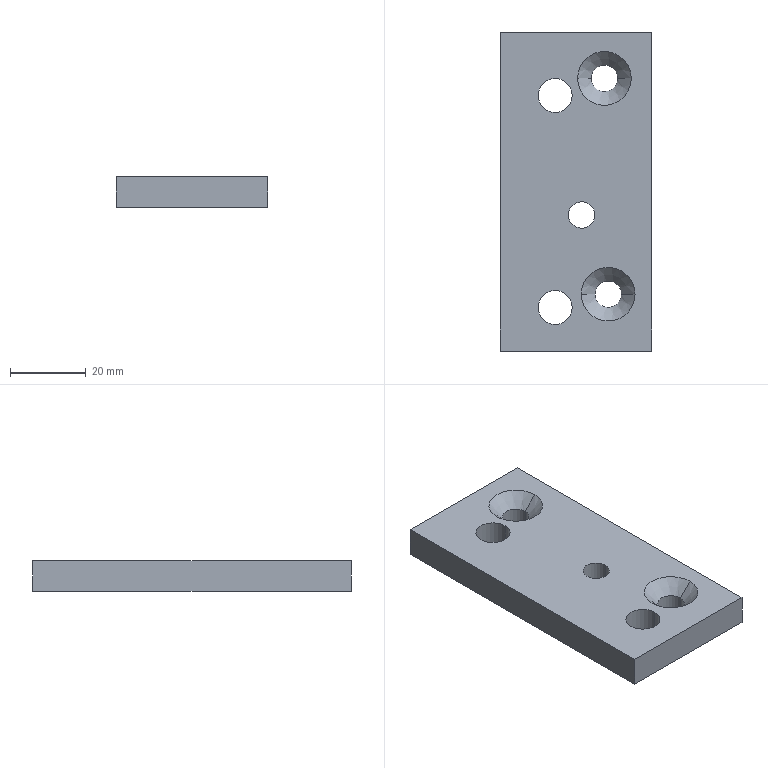Part | 1 solid | 20 faces | box 40 x 84 x 8 mm | volume 24556 mm3 | cylinder 10 | plane 6 | cone 4 | commonest cylinder face diameters 7 x6 9 x4
STEP:
#1=CARTESIAN_POINT('',(0.,0.,0.));
#2=DIRECTION('',(0.,0.,1.));
#3=DIRECTION('',(1.,0.,0.));
#4=AXIS2_PLACEMENT_3D('',#1,#2,#3);
#5=CARTESIAN_POINT('',(-251.148,521.,-248.55));
#6=VERTEX_POINT('',#5);
#7=CARTESIAN_POINT('',(-291.148,521.,-248.55));
#8=VERTEX_POINT('',#7);
#9=CARTESIAN_POINT('',(-251.148,521.,-248.55));
#10=DIRECTION('',(-1.,0.,0.));
#11=VECTOR('',#10,1.);
#12=LINE('',#9,#11);
#13=CARTESIAN_POINT('',(-251.148,521.,-256.55));
#14=DIRECTION('',(0.,1.,0.));
#15=DIRECTION('',(0.,0.,-1.));
#16=AXIS2_PLACEMENT_3D('',#13,#14,#15);
#17=PLANE('',#16);
#18=CARTESIAN_POINT('',(-8.,0.));
#19=DIRECTION('',(0.,1.));
#20=VECTOR('',#19,1.);
#21=LINE('',#18,#20);
#22=(GEOMETRIC_REPRESENTATION_CONTEXT(2)PARAMETRIC_REPRESENTATION_CONTEXT()REPRESENTATION_CONTEXT('',''));
#23=DEFINITIONAL_REPRESENTATION('',(#21),#22);
#24=PCURVE('',#17,#23);
#25=CARTESIAN_POINT('',(-276.648,504.5,-248.55));
#26=DIRECTION('',(0.,0.,1.));
#27=DIRECTION('',(-1.,0.,0.));
#28=AXIS2_PLACEMENT_3D('',#25,#26,#27);
#29=PLANE('',#28);
#30=CARTESIAN_POINT('',(-25.5,-16.5));
#31=DIRECTION('',(1.,0.));
#32=VECTOR('',#31,1.);
#33=LINE('',#30,#32);
#34=(GEOMETRIC_REPRESENTATION_CONTEXT(2)PARAMETRIC_REPRESENTATION_CONTEXT()REPRESENTATION_CONTEXT('',''));
#35=DEFINITIONAL_REPRESENTATION('',(#33),#34);
#36=PCURVE('',#29,#35);
#37=SURFACE_CURVE('',#12,(#24,#36),.PCURVE_S1.);
#38=EDGE_CURVE('',#6,#8,#37,.T.);
#39=ORIENTED_EDGE('',*,*,#38,.F.);
#40=CARTESIAN_POINT('',(-251.148,521.,-256.55));
#41=VERTEX_POINT('',#40);
#42=CARTESIAN_POINT('',(-251.148,521.,-256.55));
#43=DIRECTION('',(0.,0.,1.));
#44=VECTOR('',#43,1.);
#45=LINE('',#42,#44);
#46=CARTESIAN_POINT('',(0.,0.));
#47=DIRECTION('',(-1.,0.));
#48=VECTOR('',#47,1.);
#49=LINE('',#46,#48);
#50=(GEOMETRIC_REPRESENTATION_CONTEXT(2)PARAMETRIC_REPRESENTATION_CONTEXT()REPRESENTATION_CONTEXT('',''));
#51=DEFINITIONAL_REPRESENTATION('',(#49),#50);
#52=PCURVE('',#17,#51);
#53=CARTESIAN_POINT('',(-251.148,437.,-256.55));
#54=DIRECTION('',(1.,0.,0.));
#55=DIRECTION('',(0.,0.,1.));
#56=AXIS2_PLACEMENT_3D('',#53,#54,#55);
#57=PLANE('',#56);
#58=CARTESIAN_POINT('',(0.,-84.));
#59=DIRECTION('',(1.,0.));
#60=VECTOR('',#59,1.);
#61=LINE('',#58,#60);
#62=(GEOMETRIC_REPRESENTATION_CONTEXT(2)PARAMETRIC_REPRESENTATION_CONTEXT()REPRESENTATION_CONTEXT('',''));
#63=DEFINITIONAL_REPRESENTATION('',(#61),#62);
#64=PCURVE('',#57,#63);
#65=SURFACE_CURVE('',#45,(#52,#64),.PCURVE_S1.);
#66=EDGE_CURVE('',#41,#6,#65,.T.);
#67=ORIENTED_EDGE('',*,*,#66,.F.);
#68=CARTESIAN_POINT('',(-291.148,521.,-256.55));
#69=VERTEX_POINT('',#68);
#70=CARTESIAN_POINT('',(-251.148,521.,-256.55));
#71=DIRECTION('',(-1.,0.,0.));
#72=VECTOR('',#71,1.);
#73=LINE('',#70,#72);
#74=CARTESIAN_POINT('',(0.,0.));
#75=DIRECTION('',(0.,1.));
#76=VECTOR('',#75,1.);
#77=LINE('',#74,#76);
#78=(GEOMETRIC_REPRESENTATION_CONTEXT(2)PARAMETRIC_REPRESENTATION_CONTEXT()REPRESENTATION_CONTEXT('',''));
#79=DEFINITIONAL_REPRESENTATION('',(#77),#78);
#80=PCURVE('',#17,#79);
#81=CARTESIAN_POINT('',(-276.648,504.5,-256.55));
#82=DIRECTION('',(0.,0.,1.));
#83=DIRECTION('',(-1.,0.,0.));
#84=AXIS2_PLACEMENT_3D('',#81,#82,#83);
#85=PLANE('',#84);
#86=CARTESIAN_POINT('',(-25.5,-16.5));
#87=DIRECTION('',(1.,0.));
#88=VECTOR('',#87,1.);
#89=LINE('',#86,#88);
#90=(GEOMETRIC_REPRESENTATION_CONTEXT(2)PARAMETRIC_REPRESENTATION_CONTEXT()REPRESENTATION_CONTEXT('',''));
#91=DEFINITIONAL_REPRESENTATION('',(#89),#90);
#92=PCURVE('',#85,#91);
#93=SURFACE_CURVE('',#73,(#80,#92),.PCURVE_S1.);
#94=EDGE_CURVE('',#41,#69,#93,.T.);
#95=ORIENTED_EDGE('',*,*,#94,.T.);
#96=CARTESIAN_POINT('',(-291.148,521.,-256.55));
#97=DIRECTION('',(0.,0.,1.));
#98=VECTOR('',#97,1.);
#99=LINE('',#96,#98);
#100=CARTESIAN_POINT('',(0.,40.));
#101=DIRECTION('',(-1.,0.));
#102=VECTOR('',#101,1.);
#103=LINE('',#100,#102);
#104=(GEOMETRIC_REPRESENTATION_CONTEXT(2)PARAMETRIC_REPRESENTATION_CONTEXT()REPRESENTATION_CONTEXT('',''));
#105=DEFINITIONAL_REPRESENTATION('',(#103),#104);
#106=PCURVE('',#17,#105);
#107=CARTESIAN_POINT('',(-291.148,521.,-256.55));
#108=DIRECTION('',(-1.,0.,0.));
#109=DIRECTION('',(0.,0.,-1.));
#110=AXIS2_PLACEMENT_3D('',#107,#108,#109);
#111=PLANE('',#110);
#112=CARTESIAN_POINT('',(0.,0.));
#113=DIRECTION('',(-1.,0.));
#114=VECTOR('',#113,1.);
#115=LINE('',#112,#114);
#116=(GEOMETRIC_REPRESENTATION_CONTEXT(2)PARAMETRIC_REPRESENTATION_CONTEXT()REPRESENTATION_CONTEXT('',''));
#117=DEFINITIONAL_REPRESENTATION('',(#115),#116);
#118=PCURVE('',#111,#117);
#119=SURFACE_CURVE('',#99,(#106,#118),.PCURVE_S1.);
#120=EDGE_CURVE('',#69,#8,#119,.T.);
#121=ORIENTED_EDGE('',*,*,#120,.T.);
#122=EDGE_LOOP('',(#39,#67,#95,#121));
#123=FACE_BOUND('',#122,.T.);
#124=ADVANCED_FACE('',(#123),#17,.T.);
#125=CARTESIAN_POINT('',(-291.148,437.,-248.55));
#126=VERTEX_POINT('',#125);
#127=CARTESIAN_POINT('',(-291.148,521.,-248.55));
#128=DIRECTION('',(0.,-1.,0.));
#129=VECTOR('',#128,1.);
#130=LINE('',#127,#129);
#131=CARTESIAN_POINT('',(-8.,0.));
#132=DIRECTION('',(0.,1.));
#133=VECTOR('',#132,1.);
#134=LINE('',#131,#133);
#135=(GEOMETRIC_REPRESENTATION_CONTEXT(2)PARAMETRIC_REPRESENTATION_CONTEXT()REPRESENTATION_CONTEXT('',''));
#136=DEFINITIONAL_REPRESENTATION('',(#134),#135);
#137=PCURVE('',#111,#136);
#138=CARTESIAN_POINT('',(14.5,-16.5));
#139=DIRECTION('',(0.,1.));
#140=VECTOR('',#139,1.);
#141=LINE('',#138,#140);
#142=(GEOMETRIC_REPRESENTATION_CONTEXT(2)PARAMETRIC_REPRESENTATION_CONTEXT()REPRESENTATION_CONTEXT('',''));
#143=DEFINITIONAL_REPRESENTATION('',(#141),#142);
#144=PCURVE('',#29,#143);
#145=SURFACE_CURVE('',#130,(#137,#144),.PCURVE_S1.);
#146=EDGE_CURVE('',#8,#126,#145,.T.);
#147=ORIENTED_EDGE('',*,*,#146,.F.);
#148=ORIENTED_EDGE('',*,*,#120,.F.);
#149=CARTESIAN_POINT('',(-291.148,437.,-256.55));
#150=VERTEX_POINT('',#149);
#151=CARTESIAN_POINT('',(-291.148,521.,-256.55));
#152=DIRECTION('',(0.,-1.,0.));
#153=VECTOR('',#152,1.);
#154=LINE('',#151,#153);
#155=CARTESIAN_POINT('',(0.,0.));
#156=DIRECTION('',(0.,1.));
#157=VECTOR('',#156,1.);
#158=LINE('',#155,#157);
#159=(GEOMETRIC_REPRESENTATION_CONTEXT(2)PARAMETRIC_REPRESENTATION_CONTEXT()REPRESENTATION_CONTEXT('',''));
#160=DEFINITIONAL_REPRESENTATION('',(#158),#159);
#161=PCURVE('',#111,#160);
#162=CARTESIAN_POINT('',(14.5,-16.5));
#163=DIRECTION('',(0.,1.));
#164=VECTOR('',#163,1.);
#165=LINE('',#162,#164);
#166=(GEOMETRIC_REPRESENTATION_CONTEXT(2)PARAMETRIC_REPRESENTATION_CONTEXT()REPRESENTATION_CONTEXT('',''));
#167=DEFINITIONAL_REPRESENTATION('',(#165),#166);
#168=PCURVE('',#85,#167);
#169=SURFACE_CURVE('',#154,(#161,#168),.PCURVE_S1.);
#170=EDGE_CURVE('',#69,#150,#169,.T.);
#171=ORIENTED_EDGE('',*,*,#170,.T.);
#172=CARTESIAN_POINT('',(-291.148,437.,-256.55));
#173=DIRECTION('',(0.,0.,1.));
#174=VECTOR('',#173,1.);
#175=LINE('',#172,#174);
#176=CARTESIAN_POINT('',(0.,84.));
#177=DIRECTION('',(-1.,0.));
#178=VECTOR('',#177,1.);
#179=LINE('',#176,#178);
#180=(GEOMETRIC_REPRESENTATION_CONTEXT(2)PARAMETRIC_REPRESENTATION_CONTEXT()REPRESENTATION_CONTEXT('',''));
#181=DEFINITIONAL_REPRESENTATION('',(#179),#180);
#182=PCURVE('',#111,#181);
#183=CARTESIAN_POINT('',(-291.148,437.,-256.55));
#184=DIRECTION('',(0.,-1.,0.));
#185=DIRECTION('',(0.,0.,1.));
#186=AXIS2_PLACEMENT_3D('',#183,#184,#185);
#187=PLANE('',#186);
#188=CARTESIAN_POINT('',(0.,0.));
#189=DIRECTION('',(1.,0.));
#190=VECTOR('',#189,1.);
#191=LINE('',#188,#190);
#192=(GEOMETRIC_REPRESENTATION_CONTEXT(2)PARAMETRIC_REPRESENTATION_CONTEXT()REPRESENTATION_CONTEXT('',''));
#193=DEFINITIONAL_REPRESENTATION('',(#191),#192);
#194=PCURVE('',#187,#193);
#195=SURFACE_CURVE('',#175,(#182,#194),.PCURVE_S1.);
#196=EDGE_CURVE('',#150,#126,#195,.T.);
#197=ORIENTED_EDGE('',*,*,#196,.T.);
#198=EDGE_LOOP('',(#147,#148,#171,#197));
#199=FACE_BOUND('',#198,.T.);
#200=ADVANCED_FACE('',(#199),#111,.T.);
#201=CARTESIAN_POINT('',(-251.148,437.,-248.55));
#202=VERTEX_POINT('',#201);
#203=CARTESIAN_POINT('',(-291.148,437.,-248.55));
#204=DIRECTION('',(1.,0.,0.));
#205=VECTOR('',#204,1.);
#206=LINE('',#203,#205);
#207=CARTESIAN_POINT('',(8.,0.));
#208=DIRECTION('',(0.,-1.));
#209=VECTOR('',#208,1.);
#210=LINE('',#207,#209);
#211=(GEOMETRIC_REPRESENTATION_CONTEXT(2)PARAMETRIC_REPRESENTATION_CONTEXT()REPRESENTATION_CONTEXT('',''));
#212=DEFINITIONAL_REPRESENTATION('',(#210),#211);
#213=PCURVE('',#187,#212);
#214=CARTESIAN_POINT('',(14.5,67.5));
#215=DIRECTION('',(-1.,0.));
#216=VECTOR('',#215,1.);
#217=LINE('',#214,#216);
#218=(GEOMETRIC_REPRESENTATION_CONTEXT(2)PARAMETRIC_REPRESENTATION_CONTEXT()REPRESENTATION_CONTEXT('',''));
#219=DEFINITIONAL_REPRESENTATION('',(#217),#218);
#220=PCURVE('',#29,#219);
#221=SURFACE_CURVE('',#206,(#213,#220),.PCURVE_S1.);
#222=EDGE_CURVE('',#126,#202,#221,.T.);
#223=ORIENTED_EDGE('',*,*,#222,.F.);
#224=ORIENTED_EDGE('',*,*,#196,.F.);
#225=CARTESIAN_POINT('',(-251.148,437.,-256.55));
#226=VERTEX_POINT('',#225);
#227=CARTESIAN_POINT('',(-291.148,437.,-256.55));
#228=DIRECTION('',(1.,0.,0.));
#229=VECTOR('',#228,1.);
#230=LINE('',#227,#229);
#231=CARTESIAN_POINT('',(0.,0.));
#232=DIRECTION('',(0.,-1.));
#233=VECTOR('',#232,1.);
#234=LINE('',#231,#233);
#235=(GEOMETRIC_REPRESENTATION_CONTEXT(2)PARAMETRIC_REPRESENTATION_CONTEXT()REPRESENTATION_CONTEXT('',''));
#236=DEFINITIONAL_REPRESENTATION('',(#234),#235);
#237=PCURVE('',#187,#236);
#238=CARTESIAN_POINT('',(14.5,67.5));
#239=DIRECTION('',(-1.,0.));
#240=VECTOR('',#239,1.);
#241=LINE('',#238,#240);
#242=(GEOMETRIC_REPRESENTATION_CONTEXT(2)PARAMETRIC_REPRESENTATION_CONTEXT()REPRESENTATION_CONTEXT('',''));
#243=DEFINITIONAL_REPRESENTATION('',(#241),#242);
#244=PCURVE('',#85,#243);
#245=SURFACE_CURVE('',#230,(#237,#244),.PCURVE_S1.);
#246=EDGE_CURVE('',#150,#226,#245,.T.);
#247=ORIENTED_EDGE('',*,*,#246,.T.);
#248=CARTESIAN_POINT('',(-251.148,437.,-256.55));
#249=DIRECTION('',(0.,0.,1.));
#250=VECTOR('',#249,1.);
#251=LINE('',#248,#250);
#252=CARTESIAN_POINT('',(0.,-40.));
#253=DIRECTION('',(1.,0.));
#254=VECTOR('',#253,1.);
#255=LINE('',#252,#254);
#256=(GEOMETRIC_REPRESENTATION_CONTEXT(2)PARAMETRIC_REPRESENTATION_CONTEXT()REPRESENTATION_CONTEXT('',''));
#257=DEFINITIONAL_REPRESENTATION('',(#255),#256);
#258=PCURVE('',#187,#257);
#259=CARTESIAN_POINT('',(0.,0.));
#260=DIRECTION('',(1.,0.));
#261=VECTOR('',#260,1.);
#262=LINE('',#259,#261);
#263=(GEOMETRIC_REPRESENTATION_CONTEXT(2)PARAMETRIC_REPRESENTATION_CONTEXT()REPRESENTATION_CONTEXT('',''));
#264=DEFINITIONAL_REPRESENTATION('',(#262),#263);
#265=PCURVE('',#57,#264);
#266=SURFACE_CURVE('',#251,(#258,#265),.PCURVE_S1.);
#267=EDGE_CURVE('',#226,#202,#266,.T.);
#268=ORIENTED_EDGE('',*,*,#267,.T.);
#269=EDGE_LOOP('',(#223,#224,#247,#268));
#270=FACE_BOUND('',#269,.T.);
#271=ADVANCED_FACE('',(#270),#187,.T.);
#272=CARTESIAN_POINT('',(-251.148,437.,-248.55));
#273=DIRECTION('',(0.,1.,0.));
#274=VECTOR('',#273,1.);
#275=LINE('',#272,#274);
#276=CARTESIAN_POINT('',(8.,0.));
#277=DIRECTION('',(0.,-1.));
#278=VECTOR('',#277,1.);
#279=LINE('',#276,#278);
#280=(GEOMETRIC_REPRESENTATION_CONTEXT(2)PARAMETRIC_REPRESENTATION_CONTEXT()REPRESENTATION_CONTEXT('',''));
#281=DEFINITIONAL_REPRESENTATION('',(#279),#280);
#282=PCURVE('',#57,#281);
#283=CARTESIAN_POINT('',(-25.5,67.5));
#284=DIRECTION('',(0.,-1.));
#285=VECTOR('',#284,1.);
#286=LINE('',#283,#285);
#287=(GEOMETRIC_REPRESENTATION_CONTEXT(2)PARAMETRIC_REPRESENTATION_CONTEXT()REPRESENTATION_CONTEXT('',''));
#288=DEFINITIONAL_REPRESENTATION('',(#286),#287);
#289=PCURVE('',#29,#288);
#290=SURFACE_CURVE('',#275,(#282,#289),.PCURVE_S1.);
#291=EDGE_CURVE('',#202,#6,#290,.T.);
#292=ORIENTED_EDGE('',*,*,#291,.F.);
#293=ORIENTED_EDGE('',*,*,#267,.F.);
#294=CARTESIAN_POINT('',(-251.148,437.,-256.55));
#295=DIRECTION('',(0.,1.,0.));
#296=VECTOR('',#295,1.);
#297=LINE('',#294,#296);
#298=CARTESIAN_POINT('',(0.,0.));
#299=DIRECTION('',(0.,-1.));
#300=VECTOR('',#299,1.);
#301=LINE('',#298,#300);
#302=(GEOMETRIC_REPRESENTATION_CONTEXT(2)PARAMETRIC_REPRESENTATION_CONTEXT()REPRESENTATION_CONTEXT('',''));
#303=DEFINITIONAL_REPRESENTATION('',(#301),#302);
#304=PCURVE('',#57,#303);
#305=CARTESIAN_POINT('',(-25.5,67.5));
#306=DIRECTION('',(0.,-1.));
#307=VECTOR('',#306,1.);
#308=LINE('',#305,#307);
#309=(GEOMETRIC_REPRESENTATION_CONTEXT(2)PARAMETRIC_REPRESENTATION_CONTEXT()REPRESENTATION_CONTEXT('',''));
#310=DEFINITIONAL_REPRESENTATION('',(#308),#309);
#311=PCURVE('',#85,#310);
#312=SURFACE_CURVE('',#297,(#304,#311),.PCURVE_S1.);
#313=EDGE_CURVE('',#226,#41,#312,.T.);
#314=ORIENTED_EDGE('',*,*,#313,.T.);
#315=ORIENTED_EDGE('',*,*,#66,.T.);
#316=EDGE_LOOP('',(#292,#293,#314,#315));
#317=FACE_BOUND('',#316,.T.);
#318=ADVANCED_FACE('',(#317),#57,.T.);
#319=CARTESIAN_POINT('',(-259.148,452.,-256.55));
#320=VERTEX_POINT('',#319);
#321=CARTESIAN_POINT('',(-266.148,452.,-256.55));
#322=VERTEX_POINT('',#321);
#323=CARTESIAN_POINT('',(-262.648,452.,-256.55));
#324=DIRECTION('',(0.,0.,1.));
#325=DIRECTION('',(1.,0.,0.));
#326=AXIS2_PLACEMENT_3D('',#323,#324,#325);
#327=CIRCLE('',#326,3.5);
#328=CARTESIAN_POINT('',(-14.,52.5));
#329=DIRECTION('',(-1.,0.));
#330=AXIS2_PLACEMENT_2D('',#328,#329);
#331=CIRCLE('',#330,3.5);
#332=(GEOMETRIC_REPRESENTATION_CONTEXT(2)PARAMETRIC_REPRESENTATION_CONTEXT()REPRESENTATION_CONTEXT('',''));
#333=DEFINITIONAL_REPRESENTATION('',(#331),#332);
#334=PCURVE('',#85,#333);
#335=CARTESIAN_POINT('',(-262.648,452.,-298.55));
#336=DIRECTION('',(0.,0.,-1.));
#337=DIRECTION('',(0.,-1.,0.));
#338=AXIS2_PLACEMENT_3D('',#335,#336,#337);
#339=CYLINDRICAL_SURFACE('',#338,3.5);
#340=CARTESIAN_POINT('',(4.712,-42.));
#341=DIRECTION('',(-1.,0.));
#342=VECTOR('',#341,1.);
#343=LINE('',#340,#342);
#344=(GEOMETRIC_REPRESENTATION_CONTEXT(2)PARAMETRIC_REPRESENTATION_CONTEXT()REPRESENTATION_CONTEXT('',''));
#345=DEFINITIONAL_REPRESENTATION('',(#343),#344);
#346=PCURVE('',#339,#345);
#347=SURFACE_CURVE('',#327,(#334,#346),.PCURVE_S1.);
#348=EDGE_CURVE('',#320,#322,#347,.T.);
#349=ORIENTED_EDGE('',*,*,#348,.T.);
#350=CARTESIAN_POINT('',(-262.648,452.,-256.55));
#351=DIRECTION('',(0.,0.,1.));
#352=DIRECTION('',(1.,0.,0.));
#353=AXIS2_PLACEMENT_3D('',#350,#351,#352);
#354=CIRCLE('',#353,3.5);
#355=CARTESIAN_POINT('',(-14.,52.5));
#356=DIRECTION('',(-1.,0.));
#357=AXIS2_PLACEMENT_2D('',#355,#356);
#358=CIRCLE('',#357,3.5);
#359=(GEOMETRIC_REPRESENTATION_CONTEXT(2)PARAMETRIC_REPRESENTATION_CONTEXT()REPRESENTATION_CONTEXT('',''));
#360=DEFINITIONAL_REPRESENTATION('',(#358),#359);
#361=PCURVE('',#85,#360);
#362=CARTESIAN_POINT('',(-262.648,452.,-298.55));
#363=DIRECTION('',(0.,0.,-1.));
#364=DIRECTION('',(0.,1.,0.));
#365=AXIS2_PLACEMENT_3D('',#362,#363,#364);
#366=CYLINDRICAL_SURFACE('',#365,3.5);
#367=CARTESIAN_POINT('',(7.854,-42.));
#368=DIRECTION('',(-1.,0.));
#369=VECTOR('',#368,1.);
#370=LINE('',#367,#369);
#371=(GEOMETRIC_REPRESENTATION_CONTEXT(2)PARAMETRIC_REPRESENTATION_CONTEXT()REPRESENTATION_CONTEXT('',''));
#372=DEFINITIONAL_REPRESENTATION('',(#370),#371);
#373=PCURVE('',#366,#372);
#374=SURFACE_CURVE('',#354,(#361,#373),.PCURVE_S1.);
#375=EDGE_CURVE('',#322,#320,#374,.T.);
#376=ORIENTED_EDGE('',*,*,#375,.T.);
#377=EDGE_LOOP('',(#349,#376));
#378=FACE_BOUND('',#377,.T.);
#379=CARTESIAN_POINT('',(-260.148,509.,-256.55));
#380=VERTEX_POINT('',#379);
#381=CARTESIAN_POINT('',(-267.148,509.,-256.55));
#382=VERTEX_POINT('',#381);
#383=CARTESIAN_POINT('',(-263.648,509.,-256.55));
#384=DIRECTION('',(0.,0.,1.));
#385=DIRECTION('',(1.,0.,0.));
#386=AXIS2_PLACEMENT_3D('',#383,#384,#385);
#387=CIRCLE('',#386,3.5);
#388=CARTESIAN_POINT('',(-13.,-4.5));
#389=DIRECTION('',(-1.,0.));
#390=AXIS2_PLACEMENT_2D('',#388,#389);
#391=CIRCLE('',#390,3.5);
#392=(GEOMETRIC_REPRESENTATION_CONTEXT(2)PARAMETRIC_REPRESENTATION_CONTEXT()REPRESENTATION_CONTEXT('',''));
#393=DEFINITIONAL_REPRESENTATION('',(#391),#392);
#394=PCURVE('',#85,#393);
#395=CARTESIAN_POINT('',(-263.648,509.,-298.55));
#396=DIRECTION('',(0.,0.,-1.));
#397=DIRECTION('',(0.,-1.,0.));
#398=AXIS2_PLACEMENT_3D('',#395,#396,#397);
#399=CYLINDRICAL_SURFACE('',#398,3.5);
#400=CARTESIAN_POINT('',(4.712,-42.));
#401=DIRECTION('',(-1.,0.));
#402=VECTOR('',#401,1.);
#403=LINE('',#400,#402);
#404=(GEOMETRIC_REPRESENTATION_CONTEXT(2)PARAMETRIC_REPRESENTATION_CONTEXT()REPRESENTATION_CONTEXT('',''));
#405=DEFINITIONAL_REPRESENTATION('',(#403),#404);
#406=PCURVE('',#399,#405);
#407=SURFACE_CURVE('',#387,(#394,#406),.PCURVE_S1.);
#408=EDGE_CURVE('',#380,#382,#407,.T.);
#409=ORIENTED_EDGE('',*,*,#408,.T.);
#410=CARTESIAN_POINT('',(-263.648,509.,-256.55));
#411=DIRECTION('',(0.,0.,1.));
#412=DIRECTION('',(1.,0.,0.));
#413=AXIS2_PLACEMENT_3D('',#410,#411,#412);
#414=CIRCLE('',#413,3.5);
#415=CARTESIAN_POINT('',(-13.,-4.5));
#416=DIRECTION('',(-1.,0.));
#417=AXIS2_PLACEMENT_2D('',#415,#416);
#418=CIRCLE('',#417,3.5);
#419=(GEOMETRIC_REPRESENTATION_CONTEXT(2)PARAMETRIC_REPRESENTATION_CONTEXT()REPRESENTATION_CONTEXT('',''));
#420=DEFINITIONAL_REPRESENTATION('',(#418),#419);
#421=PCURVE('',#85,#420);
#422=CARTESIAN_POINT('',(-263.648,509.,-298.55));
#423=DIRECTION('',(0.,0.,-1.));
#424=DIRECTION('',(0.,1.,0.));
#425=AXIS2_PLACEMENT_3D('',#422,#423,#424);
#426=CYLINDRICAL_SURFACE('',#425,3.5);
#427=CARTESIAN_POINT('',(7.854,-42.));
#428=DIRECTION('',(-1.,0.));
#429=VECTOR('',#428,1.);
#430=LINE('',#427,#429);
#431=(GEOMETRIC_REPRESENTATION_CONTEXT(2)PARAMETRIC_REPRESENTATION_CONTEXT()REPRESENTATION_CONTEXT('',''));
#432=DEFINITIONAL_REPRESENTATION('',(#430),#431);
#433=PCURVE('',#426,#432);
#434=SURFACE_CURVE('',#414,(#421,#433),.PCURVE_S1.);
#435=EDGE_CURVE('',#382,#380,#434,.T.);
#436=ORIENTED_EDGE('',*,*,#435,.T.);
#437=EDGE_LOOP('',(#409,#436));
#438=FACE_BOUND('',#437,.T.);
#439=ORIENTED_EDGE('',*,*,#94,.F.);
#440=ORIENTED_EDGE('',*,*,#313,.F.);
#441=ORIENTED_EDGE('',*,*,#246,.F.);
#442=ORIENTED_EDGE('',*,*,#170,.F.);
#443=EDGE_LOOP('',(#439,#440,#441,#442));
#444=FACE_BOUND('',#443,.T.);
#445=CARTESIAN_POINT('',(-281.148,504.5,-256.55));
#446=VERTEX_POINT('',#445);
#447=CARTESIAN_POINT('',(-272.148,504.5,-256.55));
#448=VERTEX_POINT('',#447);
#449=CARTESIAN_POINT('',(-276.648,504.5,-256.55));
#450=DIRECTION('',(0.,0.,1.));
#451=DIRECTION('',(-1.,0.,0.));
#452=AXIS2_PLACEMENT_3D('',#449,#450,#451);
#453=CIRCLE('',#452,4.5);
#454=CARTESIAN_POINT('',(0.,0.));
#455=DIRECTION('',(1.,0.));
#456=AXIS2_PLACEMENT_2D('',#454,#455);
#457=CIRCLE('',#456,4.5);
#458=(GEOMETRIC_REPRESENTATION_CONTEXT(2)PARAMETRIC_REPRESENTATION_CONTEXT()REPRESENTATION_CONTEXT('',''));
#459=DEFINITIONAL_REPRESENTATION('',(#457),#458);
#460=PCURVE('',#85,#459);
#461=CARTESIAN_POINT('',(-276.648,504.5,-256.55));
#462=DIRECTION('',(0.,0.,1.));
#463=DIRECTION('',(0.,1.,0.));
#464=AXIS2_PLACEMENT_3D('',#461,#462,#463);
#465=CYLINDRICAL_SURFACE('',#464,4.5);
#466=CARTESIAN_POINT('',(1.571,0.));
#467=DIRECTION('',(1.,0.));
#468=VECTOR('',#467,1.);
#469=LINE('',#466,#468);
#470=(GEOMETRIC_REPRESENTATION_CONTEXT(2)PARAMETRIC_REPRESENTATION_CONTEXT()REPRESENTATION_CONTEXT('',''));
#471=DEFINITIONAL_REPRESENTATION('',(#469),#470);
#472=PCURVE('',#465,#471);
#473=SURFACE_CURVE('',#453,(#460,#472),.PCURVE_S1.);
#474=EDGE_CURVE('',#446,#448,#473,.T.);
#475=ORIENTED_EDGE('',*,*,#474,.T.);
#476=CARTESIAN_POINT('',(-276.648,504.5,-256.55));
#477=DIRECTION('',(0.,0.,1.));
#478=DIRECTION('',(-1.,0.,0.));
#479=AXIS2_PLACEMENT_3D('',#476,#477,#478);
#480=CIRCLE('',#479,4.5);
#481=CARTESIAN_POINT('',(0.,0.));
#482=DIRECTION('',(1.,0.));
#483=AXIS2_PLACEMENT_2D('',#481,#482);
#484=CIRCLE('',#483,4.5);
#485=(GEOMETRIC_REPRESENTATION_CONTEXT(2)PARAMETRIC_REPRESENTATION_CONTEXT()REPRESENTATION_CONTEXT('',''));
#486=DEFINITIONAL_REPRESENTATION('',(#484),#485);
#487=PCURVE('',#85,#486);
#488=CARTESIAN_POINT('',(-276.648,504.5,-256.55));
#489=DIRECTION('',(0.,0.,1.));
#490=DIRECTION('',(0.,-1.,0.));
#491=AXIS2_PLACEMENT_3D('',#488,#489,#490);
#492=CYLINDRICAL_SURFACE('',#491,4.5);
#493=CARTESIAN_POINT('',(-1.571,0.));
#494=DIRECTION('',(1.,0.));
#495=VECTOR('',#494,1.);
#496=LINE('',#493,#495);
#497=(GEOMETRIC_REPRESENTATION_CONTEXT(2)PARAMETRIC_REPRESENTATION_CONTEXT()REPRESENTATION_CONTEXT('',''));
#498=DEFINITIONAL_REPRESENTATION('',(#496),#497);
#499=PCURVE('',#492,#498);
#500=SURFACE_CURVE('',#480,(#487,#499),.PCURVE_S1.);
#501=EDGE_CURVE('',#448,#446,#500,.T.);
#502=ORIENTED_EDGE('',*,*,#501,.T.);
#503=EDGE_LOOP('',(#475,#502));
#504=FACE_BOUND('',#503,.T.);
#505=CARTESIAN_POINT('',(-273.148,472.924,-256.55));
#506=VERTEX_POINT('',#505);
#507=CARTESIAN_POINT('',(-266.148,472.924,-256.55));
#508=VERTEX_POINT('',#507);
#509=CARTESIAN_POINT('',(-269.648,472.924,-256.55));
#510=DIRECTION('',(0.,0.,1.));
#511=DIRECTION('',(-1.,0.,0.));
#512=AXIS2_PLACEMENT_3D('',#509,#510,#511);
#513=CIRCLE('',#512,3.5);
#514=CARTESIAN_POINT('',(-7.,31.576));
#515=DIRECTION('',(1.,0.));
#516=AXIS2_PLACEMENT_2D('',#514,#515);
#517=CIRCLE('',#516,3.5);
#518=(GEOMETRIC_REPRESENTATION_CONTEXT(2)PARAMETRIC_REPRESENTATION_CONTEXT()REPRESENTATION_CONTEXT('',''));
#519=DEFINITIONAL_REPRESENTATION('',(#517),#518);
#520=PCURVE('',#85,#519);
#521=CARTESIAN_POINT('',(-269.648,472.924,-256.55));
#522=DIRECTION('',(0.,0.,1.));
#523=DIRECTION('',(0.,1.,0.));
#524=AXIS2_PLACEMENT_3D('',#521,#522,#523);
#525=CYLINDRICAL_SURFACE('',#524,3.5);
#526=CARTESIAN_POINT('',(1.571,0.));
#527=DIRECTION('',(1.,0.));
#528=VECTOR('',#527,1.);
#529=LINE('',#526,#528);
#530=(GEOMETRIC_REPRESENTATION_CONTEXT(2)PARAMETRIC_REPRESENTATION_CONTEXT()REPRESENTATION_CONTEXT('',''));
#531=DEFINITIONAL_REPRESENTATION('',(#529),#530);
#532=PCURVE('',#525,#531);
#533=SURFACE_CURVE('',#513,(#520,#532),.PCURVE_S1.);
#534=EDGE_CURVE('',#506,#508,#533,.T.);
#535=ORIENTED_EDGE('',*,*,#534,.T.);
#536=CARTESIAN_POINT('',(-269.648,472.924,-256.55));
#537=DIRECTION('',(0.,0.,1.));
#538=DIRECTION('',(-1.,0.,0.));
#539=AXIS2_PLACEMENT_3D('',#536,#537,#538);
#540=CIRCLE('',#539,3.5);
#541=CARTESIAN_POINT('',(-7.,31.576));
#542=DIRECTION('',(1.,0.));
#543=AXIS2_PLACEMENT_2D('',#541,#542);
#544=CIRCLE('',#543,3.5);
#545=(GEOMETRIC_REPRESENTATION_CONTEXT(2)PARAMETRIC_REPRESENTATION_CONTEXT()REPRESENTATION_CONTEXT('',''));
#546=DEFINITIONAL_REPRESENTATION('',(#544),#545);
#547=PCURVE('',#85,#546);
#548=CARTESIAN_POINT('',(-269.648,472.924,-256.55));
#549=DIRECTION('',(0.,0.,1.));
#550=DIRECTION('',(0.,-1.,0.));
#551=AXIS2_PLACEMENT_3D('',#548,#549,#550);
#552=CYLINDRICAL_SURFACE('',#551,3.5);
#553=CARTESIAN_POINT('',(-1.571,0.));
#554=DIRECTION('',(1.,0.));
#555=VECTOR('',#554,1.);
#556=LINE('',#553,#555);
#557=(GEOMETRIC_REPRESENTATION_CONTEXT(2)PARAMETRIC_REPRESENTATION_CONTEXT()REPRESENTATION_CONTEXT('',''));
#558=DEFINITIONAL_REPRESENTATION('',(#556),#557);
#559=PCURVE('',#552,#558);
#560=SURFACE_CURVE('',#540,(#547,#559),.PCURVE_S1.);
#561=EDGE_CURVE('',#508,#506,#560,.T.);
#562=ORIENTED_EDGE('',*,*,#561,.T.);
#563=EDGE_LOOP('',(#535,#562));
#564=FACE_BOUND('',#563,.T.);
#565=CARTESIAN_POINT('',(-281.148,448.5,-256.55));
#566=VERTEX_POINT('',#565);
#567=CARTESIAN_POINT('',(-272.148,448.5,-256.55));
#568=VERTEX_POINT('',#567);
#569=CARTESIAN_POINT('',(-276.648,448.5,-256.55));
#570=DIRECTION('',(0.,0.,1.));
#571=DIRECTION('',(-1.,0.,0.));
#572=AXIS2_PLACEMENT_3D('',#569,#570,#571);
#573=CIRCLE('',#572,4.5);
#574=CARTESIAN_POINT('',(0.,56.));
#575=DIRECTION('',(1.,0.));
#576=AXIS2_PLACEMENT_2D('',#574,#575);
#577=CIRCLE('',#576,4.5);
#578=(GEOMETRIC_REPRESENTATION_CONTEXT(2)PARAMETRIC_REPRESENTATION_CONTEXT()REPRESENTATION_CONTEXT('',''));
#579=DEFINITIONAL_REPRESENTATION('',(#577),#578);
#580=PCURVE('',#85,#579);
#581=CARTESIAN_POINT('',(-276.648,448.5,-256.55));
#582=DIRECTION('',(0.,0.,1.));
#583=DIRECTION('',(0.,1.,0.));
#584=AXIS2_PLACEMENT_3D('',#581,#582,#583);
#585=CYLINDRICAL_SURFACE('',#584,4.5);
#586=CARTESIAN_POINT('',(1.571,0.));
#587=DIRECTION('',(1.,0.));
#588=VECTOR('',#587,1.);
#589=LINE('',#586,#588);
#590=(GEOMETRIC_REPRESENTATION_CONTEXT(2)PARAMETRIC_REPRESENTATION_CONTEXT()REPRESENTATION_CONTEXT('',''));
#591=DEFINITIONAL_REPRESENTATION('',(#589),#590);
#592=PCURVE('',#585,#591);
#593=SURFACE_CURVE('',#573,(#580,#592),.PCURVE_S1.);
#594=EDGE_CURVE('',#566,#568,#593,.T.);
#595=ORIENTED_EDGE('',*,*,#594,.T.);
#596=CARTESIAN_POINT('',(-276.648,448.5,-256.55));
#597=DIRECTION('',(0.,0.,1.));
#598=DIRECTION('',(-1.,0.,0.));
#599=AXIS2_PLACEMENT_3D('',#596,#597,#598);
#600=CIRCLE('',#599,4.5);
#601=CARTESIAN_POINT('',(0.,56.));
#602=DIRECTION('',(1.,0.));
#603=AXIS2_PLACEMENT_2D('',#601,#602);
#604=CIRCLE('',#603,4.5);
#605=(GEOMETRIC_REPRESENTATION_CONTEXT(2)PARAMETRIC_REPRESENTATION_CONTEXT()REPRESENTATION_CONTEXT('',''));
#606=DEFINITIONAL_REPRESENTATION('',(#604),#605);
#607=PCURVE('',#85,#606);
#608=CARTESIAN_POINT('',(-276.648,448.5,-256.55));
#609=DIRECTION('',(0.,0.,1.));
#610=DIRECTION('',(0.,-1.,0.));
#611=AXIS2_PLACEMENT_3D('',#608,#609,#610);
#612=CYLINDRICAL_SURFACE('',#611,4.5);
#613=CARTESIAN_POINT('',(-1.571,0.));
#614=DIRECTION('',(1.,0.));
#615=VECTOR('',#614,1.);
#616=LINE('',#613,#615);
#617=(GEOMETRIC_REPRESENTATION_CONTEXT(2)PARAMETRIC_REPRESENTATION_CONTEXT()REPRESENTATION_CONTEXT('',''));
#618=DEFINITIONAL_REPRESENTATION('',(#616),#617);
#619=PCURVE('',#612,#618);
#620=SURFACE_CURVE('',#600,(#607,#619),.PCURVE_S1.);
#621=EDGE_CURVE('',#568,#566,#620,.T.);
#622=ORIENTED_EDGE('',*,*,#621,.T.);
#623=EDGE_LOOP('',(#595,#622));
#624=FACE_BOUND('',#623,.T.);
#625=ADVANCED_FACE('',(#378,#438,#444,#504,#564,#624),#85,.F.);
#626=ORIENTED_EDGE('',*,*,#621,.T.);
#627=CARTESIAN_POINT('',(-281.148,448.5,-248.55));
#628=VERTEX_POINT('',#627);
#629=CARTESIAN_POINT('',(-281.148,448.5,-256.55));
#630=DIRECTION('',(0.,0.,1.));
#631=VECTOR('',#630,1.);
#632=LINE('',#629,#631);
#633=CARTESIAN_POINT('',(4.712,0.));
#634=DIRECTION('',(0.,1.));
#635=VECTOR('',#634,1.);
#636=LINE('',#633,#635);
#637=(GEOMETRIC_REPRESENTATION_CONTEXT(2)PARAMETRIC_REPRESENTATION_CONTEXT()REPRESENTATION_CONTEXT('',''));
#638=DEFINITIONAL_REPRESENTATION('',(#636),#637);
#639=PCURVE('',#612,#638);
#640=CARTESIAN_POINT('',(1.571,0.));
#641=DIRECTION('',(0.,1.));
#642=VECTOR('',#641,1.);
#643=LINE('',#640,#642);
#644=(GEOMETRIC_REPRESENTATION_CONTEXT(2)PARAMETRIC_REPRESENTATION_CONTEXT()REPRESENTATION_CONTEXT('',''));
#645=DEFINITIONAL_REPRESENTATION('',(#643),#644);
#646=PCURVE('',#585,#645);
#647=SURFACE_CURVE('',#632,(#639,#646),.PCURVE_S1.);
#648=EDGE_CURVE('',#566,#628,#647,.T.);
#649=ORIENTED_EDGE('',*,*,#648,.T.);
#650=CARTESIAN_POINT('',(-272.148,448.5,-248.55));
#651=VERTEX_POINT('',#650);
#652=CARTESIAN_POINT('',(-276.648,448.5,-248.55));
#653=DIRECTION('',(0.,0.,1.));
#654=DIRECTION('',(-1.,0.,0.));
#655=AXIS2_PLACEMENT_3D('',#652,#653,#654);
#656=CIRCLE('',#655,4.5);
#657=CARTESIAN_POINT('',(-1.571,8.));
#658=DIRECTION('',(1.,0.));
#659=VECTOR('',#658,1.);
#660=LINE('',#657,#659);
#661=(GEOMETRIC_REPRESENTATION_CONTEXT(2)PARAMETRIC_REPRESENTATION_CONTEXT()REPRESENTATION_CONTEXT('',''));
#662=DEFINITIONAL_REPRESENTATION('',(#660),#661);
#663=PCURVE('',#612,#662);
#664=CARTESIAN_POINT('',(0.,56.));
#665=DIRECTION('',(1.,0.));
#666=AXIS2_PLACEMENT_2D('',#664,#665);
#667=CIRCLE('',#666,4.5);
#668=(GEOMETRIC_REPRESENTATION_CONTEXT(2)PARAMETRIC_REPRESENTATION_CONTEXT()REPRESENTATION_CONTEXT('',''));
#669=DEFINITIONAL_REPRESENTATION('',(#667),#668);
#670=PCURVE('',#29,#669);
#671=SURFACE_CURVE('',#656,(#663,#670),.PCURVE_S1.);
#672=EDGE_CURVE('',#651,#628,#671,.T.);
#673=ORIENTED_EDGE('',*,*,#672,.F.);
#674=CARTESIAN_POINT('',(-272.148,448.5,-256.55));
#675=DIRECTION('',(0.,0.,1.));
#676=VECTOR('',#675,1.);
#677=LINE('',#674,#676);
#678=CARTESIAN_POINT('',(1.571,0.));
#679=DIRECTION('',(0.,1.));
#680=VECTOR('',#679,1.);
#681=LINE('',#678,#680);
#682=(GEOMETRIC_REPRESENTATION_CONTEXT(2)PARAMETRIC_REPRESENTATION_CONTEXT()REPRESENTATION_CONTEXT('',''));
#683=DEFINITIONAL_REPRESENTATION('',(#681),#682);
#684=PCURVE('',#612,#683);
#685=CARTESIAN_POINT('',(4.712,0.));
#686=DIRECTION('',(0.,1.));
#687=VECTOR('',#686,1.);
#688=LINE('',#685,#687);
#689=(GEOMETRIC_REPRESENTATION_CONTEXT(2)PARAMETRIC_REPRESENTATION_CONTEXT()REPRESENTATION_CONTEXT('',''));
#690=DEFINITIONAL_REPRESENTATION('',(#688),#689);
#691=PCURVE('',#585,#690);
#692=SURFACE_CURVE('',#677,(#684,#691),.PCURVE_S1.);
#693=EDGE_CURVE('',#568,#651,#692,.T.);
#694=ORIENTED_EDGE('',*,*,#693,.F.);
#695=EDGE_LOOP('',(#626,#649,#673,#694));
#696=FACE_BOUND('',#695,.F.);
#697=ADVANCED_FACE('',(#696),#612,.F.);
#698=CARTESIAN_POINT('',(-269.748,452.,-248.55));
#699=VERTEX_POINT('',#698);
#700=CARTESIAN_POINT('',(-255.548,452.,-248.55));
#701=VERTEX_POINT('',#700);
#702=CARTESIAN_POINT('',(-262.648,452.,-248.55));
#703=DIRECTION('',(0.,0.,-1.));
#704=DIRECTION('',(-1.,0.,0.));
#705=AXIS2_PLACEMENT_3D('',#702,#703,#704);
#706=CIRCLE('',#705,7.1);
#707=CARTESIAN_POINT('',(-6.9,52.5));
#708=CARTESIAN_POINT('',(-6.9,40.203));
#709=CARTESIAN_POINT('',(-17.55,46.351));
#710=CARTESIAN_POINT('',(-28.2,52.5));
#711=CARTESIAN_POINT('',(-17.55,58.649));
#712=CARTESIAN_POINT('',(-6.9,64.798));
#713=CARTESIAN_POINT('',(-6.9,52.5));
#714=(BOUNDED_CURVE()B_SPLINE_CURVE(2,(#707,#708,#709,#710,#711,#712,#713),.UNSPECIFIED.,.T.,.F.)B_SPLINE_CURVE_WITH_KNOTS((1,2,2,2,2,1),(-2.094,0.,2.094,4.189,6.283,8.378),.UNSPECIFIED.)CURVE()GEOMETRIC_REPRESENTATION_ITEM()RATIONAL_B_SPLINE_CURVE((1.,0.5,1.,0.5,1.,0.5,1.))REPRESENTATION_ITEM(''));
#715=(GEOMETRIC_REPRESENTATION_CONTEXT(2)PARAMETRIC_REPRESENTATION_CONTEXT()REPRESENTATION_CONTEXT('',''));
#716=DEFINITIONAL_REPRESENTATION('',(#714),#715);
#717=PCURVE('',#29,#716);
#718=CARTESIAN_POINT('',(-262.648,452.,-248.55));
#719=DIRECTION('',(0.,0.,1.));
#720=DIRECTION('',(0.,-1.,0.));
#721=AXIS2_PLACEMENT_3D('',#718,#719,#720);
#722=CONICAL_SURFACE('',#721,7.1,0.7854);
#723=CARTESIAN_POINT('',(4.712,0.));
#724=DIRECTION('',(-1.,0.));
#725=VECTOR('',#724,1.);
#726=LINE('',#723,#725);
#727=(GEOMETRIC_REPRESENTATION_CONTEXT(2)PARAMETRIC_REPRESENTATION_CONTEXT()REPRESENTATION_CONTEXT('',''));
#728=DEFINITIONAL_REPRESENTATION('',(#726),#727);
#729=PCURVE('',#722,#728);
#730=SURFACE_CURVE('',#706,(#717,#729),.PCURVE_S1.);
#731=EDGE_CURVE('',#699,#701,#730,.T.);
#732=ORIENTED_EDGE('',*,*,#731,.T.);
#733=CARTESIAN_POINT('',(-262.648,452.,-248.55));
#734=DIRECTION('',(0.,0.,-1.));
#735=DIRECTION('',(-1.,0.,0.));
#736=AXIS2_PLACEMENT_3D('',#733,#734,#735);
#737=CIRCLE('',#736,7.1);
#738=CARTESIAN_POINT('',(-6.9,52.5));
#739=CARTESIAN_POINT('',(-6.9,40.203));
#740=CARTESIAN_POINT('',(-17.55,46.351));
#741=CARTESIAN_POINT('',(-28.2,52.5));
#742=CARTESIAN_POINT('',(-17.55,58.649));
#743=CARTESIAN_POINT('',(-6.9,64.798));
#744=CARTESIAN_POINT('',(-6.9,52.5));
#745=(BOUNDED_CURVE()B_SPLINE_CURVE(2,(#738,#739,#740,#741,#742,#743,#744),.UNSPECIFIED.,.T.,.F.)B_SPLINE_CURVE_WITH_KNOTS((1,2,2,2,2,1),(-2.094,0.,2.094,4.189,6.283,8.378),.UNSPECIFIED.)CURVE()GEOMETRIC_REPRESENTATION_ITEM()RATIONAL_B_SPLINE_CURVE((1.,0.5,1.,0.5,1.,0.5,1.))REPRESENTATION_ITEM(''));
#746=(GEOMETRIC_REPRESENTATION_CONTEXT(2)PARAMETRIC_REPRESENTATION_CONTEXT()REPRESENTATION_CONTEXT('',''));
#747=DEFINITIONAL_REPRESENTATION('',(#745),#746);
#748=PCURVE('',#29,#747);
#749=CARTESIAN_POINT('',(-262.648,452.,-248.55));
#750=DIRECTION('',(0.,0.,1.));
#751=DIRECTION('',(0.,1.,0.));
#752=AXIS2_PLACEMENT_3D('',#749,#750,#751);
#753=CONICAL_SURFACE('',#752,7.1,0.7854);
#754=CARTESIAN_POINT('',(7.854,0.));
#755=DIRECTION('',(-1.,0.));
#756=VECTOR('',#755,1.);
#757=LINE('',#754,#756);
#758=(GEOMETRIC_REPRESENTATION_CONTEXT(2)PARAMETRIC_REPRESENTATION_CONTEXT()REPRESENTATION_CONTEXT('',''));
#759=DEFINITIONAL_REPRESENTATION('',(#757),#758);
#760=PCURVE('',#753,#759);
#761=SURFACE_CURVE('',#737,(#748,#760),.PCURVE_S1.);
#762=EDGE_CURVE('',#701,#699,#761,.T.);
#763=ORIENTED_EDGE('',*,*,#762,.T.);
#764=EDGE_LOOP('',(#732,#763));
#765=FACE_BOUND('',#764,.T.);
#766=CARTESIAN_POINT('',(-270.748,509.,-248.55));
#767=VERTEX_POINT('',#766);
#768=CARTESIAN_POINT('',(-256.548,509.,-248.55));
#769=VERTEX_POINT('',#768);
#770=CARTESIAN_POINT('',(-263.648,509.,-248.55));
#771=DIRECTION('',(0.,0.,-1.));
#772=DIRECTION('',(-1.,0.,0.));
#773=AXIS2_PLACEMENT_3D('',#770,#771,#772);
#774=CIRCLE('',#773,7.1);
#775=CARTESIAN_POINT('',(-5.9,-4.5));
#776=CARTESIAN_POINT('',(-5.9,-16.798));
#777=CARTESIAN_POINT('',(-16.55,-10.649));
#778=CARTESIAN_POINT('',(-27.2,-4.5));
#779=CARTESIAN_POINT('',(-16.55,1.649));
#780=CARTESIAN_POINT('',(-5.9,7.798));
#781=CARTESIAN_POINT('',(-5.9,-4.5));
#782=(BOUNDED_CURVE()B_SPLINE_CURVE(2,(#775,#776,#777,#778,#779,#780,#781),.UNSPECIFIED.,.T.,.F.)B_SPLINE_CURVE_WITH_KNOTS((1,2,2,2,2,1),(-2.094,0.,2.094,4.189,6.283,8.378),.UNSPECIFIED.)CURVE()GEOMETRIC_REPRESENTATION_ITEM()RATIONAL_B_SPLINE_CURVE((1.,0.5,1.,0.5,1.,0.5,1.))REPRESENTATION_ITEM(''));
#783=(GEOMETRIC_REPRESENTATION_CONTEXT(2)PARAMETRIC_REPRESENTATION_CONTEXT()REPRESENTATION_CONTEXT('',''));
#784=DEFINITIONAL_REPRESENTATION('',(#782),#783);
#785=PCURVE('',#29,#784);
#786=CARTESIAN_POINT('',(-263.648,509.,-248.55));
#787=DIRECTION('',(0.,0.,1.));
#788=DIRECTION('',(0.,-1.,0.));
#789=AXIS2_PLACEMENT_3D('',#786,#787,#788);
#790=CONICAL_SURFACE('',#789,7.1,0.7854);
#791=CARTESIAN_POINT('',(4.712,0.));
#792=DIRECTION('',(-1.,0.));
#793=VECTOR('',#792,1.);
#794=LINE('',#791,#793);
#795=(GEOMETRIC_REPRESENTATION_CONTEXT(2)PARAMETRIC_REPRESENTATION_CONTEXT()REPRESENTATION_CONTEXT('',''));
#796=DEFINITIONAL_REPRESENTATION('',(#794),#795);
#797=PCURVE('',#790,#796);
#798=SURFACE_CURVE('',#774,(#785,#797),.PCURVE_S1.);
#799=EDGE_CURVE('',#767,#769,#798,.T.);
#800=ORIENTED_EDGE('',*,*,#799,.T.);
#801=CARTESIAN_POINT('',(-263.648,509.,-248.55));
#802=DIRECTION('',(0.,0.,-1.));
#803=DIRECTION('',(-1.,0.,0.));
#804=AXIS2_PLACEMENT_3D('',#801,#802,#803);
#805=CIRCLE('',#804,7.1);
#806=CARTESIAN_POINT('',(-5.9,-4.5));
#807=CARTESIAN_POINT('',(-5.9,-16.798));
#808=CARTESIAN_POINT('',(-16.55,-10.649));
#809=CARTESIAN_POINT('',(-27.2,-4.5));
#810=CARTESIAN_POINT('',(-16.55,1.649));
#811=CARTESIAN_POINT('',(-5.9,7.798));
#812=CARTESIAN_POINT('',(-5.9,-4.5));
#813=(BOUNDED_CURVE()B_SPLINE_CURVE(2,(#806,#807,#808,#809,#810,#811,#812),.UNSPECIFIED.,.T.,.F.)B_SPLINE_CURVE_WITH_KNOTS((1,2,2,2,2,1),(-2.094,0.,2.094,4.189,6.283,8.378),.UNSPECIFIED.)CURVE()GEOMETRIC_REPRESENTATION_ITEM()RATIONAL_B_SPLINE_CURVE((1.,0.5,1.,0.5,1.,0.5,1.))REPRESENTATION_ITEM(''));
#814=(GEOMETRIC_REPRESENTATION_CONTEXT(2)PARAMETRIC_REPRESENTATION_CONTEXT()REPRESENTATION_CONTEXT('',''));
#815=DEFINITIONAL_REPRESENTATION('',(#813),#814);
#816=PCURVE('',#29,#815);
#817=CARTESIAN_POINT('',(-263.648,509.,-248.55));
#818=DIRECTION('',(0.,0.,1.));
#819=DIRECTION('',(0.,1.,0.));
#820=AXIS2_PLACEMENT_3D('',#817,#818,#819);
#821=CONICAL_SURFACE('',#820,7.1,0.7854);
#822=CARTESIAN_POINT('',(7.854,0.));
#823=DIRECTION('',(-1.,0.));
#824=VECTOR('',#823,1.);
#825=LINE('',#822,#824);
#826=(GEOMETRIC_REPRESENTATION_CONTEXT(2)PARAMETRIC_REPRESENTATION_CONTEXT()REPRESENTATION_CONTEXT('',''));
#827=DEFINITIONAL_REPRESENTATION('',(#825),#826);
#828=PCURVE('',#821,#827);
#829=SURFACE_CURVE('',#805,(#816,#828),.PCURVE_S1.);
#830=EDGE_CURVE('',#769,#767,#829,.T.);
#831=ORIENTED_EDGE('',*,*,#830,.T.);
#832=EDGE_LOOP('',(#800,#831));
#833=FACE_BOUND('',#832,.T.);
#834=ORIENTED_EDGE('',*,*,#38,.T.);
#835=ORIENTED_EDGE('',*,*,#146,.T.);
#836=ORIENTED_EDGE('',*,*,#222,.T.);
#837=ORIENTED_EDGE('',*,*,#291,.T.);
#838=EDGE_LOOP('',(#834,#835,#836,#837));
#839=FACE_BOUND('',#838,.T.);
#840=CARTESIAN_POINT('',(-272.148,504.5,-248.55));
#841=VERTEX_POINT('',#840);
#842=CARTESIAN_POINT('',(-281.148,504.5,-248.55));
#843=VERTEX_POINT('',#842);
#844=CARTESIAN_POINT('',(-276.648,504.5,-248.55));
#845=DIRECTION('',(0.,0.,1.));
#846=DIRECTION('',(-1.,0.,0.));
#847=AXIS2_PLACEMENT_3D('',#844,#845,#846);
#848=CIRCLE('',#847,4.5);
#849=CARTESIAN_POINT('',(0.,0.));
#850=DIRECTION('',(1.,0.));
#851=AXIS2_PLACEMENT_2D('',#849,#850);
#852=CIRCLE('',#851,4.5);
#853=(GEOMETRIC_REPRESENTATION_CONTEXT(2)PARAMETRIC_REPRESENTATION_CONTEXT()REPRESENTATION_CONTEXT('',''));
#854=DEFINITIONAL_REPRESENTATION('',(#852),#853);
#855=PCURVE('',#29,#854);
#856=CARTESIAN_POINT('',(-1.571,8.));
#857=DIRECTION('',(1.,0.));
#858=VECTOR('',#857,1.);
#859=LINE('',#856,#858);
#860=(GEOMETRIC_REPRESENTATION_CONTEXT(2)PARAMETRIC_REPRESENTATION_CONTEXT()REPRESENTATION_CONTEXT('',''));
#861=DEFINITIONAL_REPRESENTATION('',(#859),#860);
#862=PCURVE('',#492,#861);
#863=SURFACE_CURVE('',#848,(#855,#862),.PCURVE_S1.);
#864=EDGE_CURVE('',#841,#843,#863,.T.);
#865=ORIENTED_EDGE('',*,*,#864,.F.);
#866=CARTESIAN_POINT('',(-276.648,504.5,-248.55));
#867=DIRECTION('',(0.,0.,1.));
#868=DIRECTION('',(-1.,0.,0.));
#869=AXIS2_PLACEMENT_3D('',#866,#867,#868);
#870=CIRCLE('',#869,4.5);
#871=CARTESIAN_POINT('',(0.,0.));
#872=DIRECTION('',(1.,0.));
#873=AXIS2_PLACEMENT_2D('',#871,#872);
#874=CIRCLE('',#873,4.5);
#875=(GEOMETRIC_REPRESENTATION_CONTEXT(2)PARAMETRIC_REPRESENTATION_CONTEXT()REPRESENTATION_CONTEXT('',''));
#876=DEFINITIONAL_REPRESENTATION('',(#874),#875);
#877=PCURVE('',#29,#876);
#878=CARTESIAN_POINT('',(1.571,8.));
#879=DIRECTION('',(1.,0.));
#880=VECTOR('',#879,1.);
#881=LINE('',#878,#880);
#882=(GEOMETRIC_REPRESENTATION_CONTEXT(2)PARAMETRIC_REPRESENTATION_CONTEXT()REPRESENTATION_CONTEXT('',''));
#883=DEFINITIONAL_REPRESENTATION('',(#881),#882);
#884=PCURVE('',#465,#883);
#885=SURFACE_CURVE('',#870,(#877,#884),.PCURVE_S1.);
#886=EDGE_CURVE('',#843,#841,#885,.T.);
#887=ORIENTED_EDGE('',*,*,#886,.F.);
#888=EDGE_LOOP('',(#865,#887));
#889=FACE_BOUND('',#888,.T.);
#890=CARTESIAN_POINT('',(-266.148,472.924,-248.55));
#891=VERTEX_POINT('',#890);
#892=CARTESIAN_POINT('',(-273.148,472.924,-248.55));
#893=VERTEX_POINT('',#892);
#894=CARTESIAN_POINT('',(-269.648,472.924,-248.55));
#895=DIRECTION('',(0.,0.,1.));
#896=DIRECTION('',(-1.,0.,0.));
#897=AXIS2_PLACEMENT_3D('',#894,#895,#896);
#898=CIRCLE('',#897,3.5);
#899=CARTESIAN_POINT('',(-7.,31.576));
#900=DIRECTION('',(1.,0.));
#901=AXIS2_PLACEMENT_2D('',#899,#900);
#902=CIRCLE('',#901,3.5);
#903=(GEOMETRIC_REPRESENTATION_CONTEXT(2)PARAMETRIC_REPRESENTATION_CONTEXT()REPRESENTATION_CONTEXT('',''));
#904=DEFINITIONAL_REPRESENTATION('',(#902),#903);
#905=PCURVE('',#29,#904);
#906=CARTESIAN_POINT('',(-1.571,8.));
#907=DIRECTION('',(1.,0.));
#908=VECTOR('',#907,1.);
#909=LINE('',#906,#908);
#910=(GEOMETRIC_REPRESENTATION_CONTEXT(2)PARAMETRIC_REPRESENTATION_CONTEXT()REPRESENTATION_CONTEXT('',''));
#911=DEFINITIONAL_REPRESENTATION('',(#909),#910);
#912=PCURVE('',#552,#911);
#913=SURFACE_CURVE('',#898,(#905,#912),.PCURVE_S1.);
#914=EDGE_CURVE('',#891,#893,#913,.T.);
#915=ORIENTED_EDGE('',*,*,#914,.F.);
#916=CARTESIAN_POINT('',(-269.648,472.924,-248.55));
#917=DIRECTION('',(0.,0.,1.));
#918=DIRECTION('',(-1.,0.,0.));
#919=AXIS2_PLACEMENT_3D('',#916,#917,#918);
#920=CIRCLE('',#919,3.5);
#921=CARTESIAN_POINT('',(-7.,31.576));
#922=DIRECTION('',(1.,0.));
#923=AXIS2_PLACEMENT_2D('',#921,#922);
#924=CIRCLE('',#923,3.5);
#925=(GEOMETRIC_REPRESENTATION_CONTEXT(2)PARAMETRIC_REPRESENTATION_CONTEXT()REPRESENTATION_CONTEXT('',''));
#926=DEFINITIONAL_REPRESENTATION('',(#924),#925);
#927=PCURVE('',#29,#926);
#928=CARTESIAN_POINT('',(1.571,8.));
#929=DIRECTION('',(1.,0.));
#930=VECTOR('',#929,1.);
#931=LINE('',#928,#930);
#932=(GEOMETRIC_REPRESENTATION_CONTEXT(2)PARAMETRIC_REPRESENTATION_CONTEXT()REPRESENTATION_CONTEXT('',''));
#933=DEFINITIONAL_REPRESENTATION('',(#931),#932);
#934=PCURVE('',#525,#933);
#935=SURFACE_CURVE('',#920,(#927,#934),.PCURVE_S1.);
#936=EDGE_CURVE('',#893,#891,#935,.T.);
#937=ORIENTED_EDGE('',*,*,#936,.F.);
#938=EDGE_LOOP('',(#915,#937));
#939=FACE_BOUND('',#938,.T.);
#940=ORIENTED_EDGE('',*,*,#672,.F.);
#941=CARTESIAN_POINT('',(-276.648,448.5,-248.55));
#942=DIRECTION('',(0.,0.,1.));
#943=DIRECTION('',(-1.,0.,0.));
#944=AXIS2_PLACEMENT_3D('',#941,#942,#943);
#945=CIRCLE('',#944,4.5);
#946=CARTESIAN_POINT('',(0.,56.));
#947=DIRECTION('',(1.,0.));
#948=AXIS2_PLACEMENT_2D('',#946,#947);
#949=CIRCLE('',#948,4.5);
#950=(GEOMETRIC_REPRESENTATION_CONTEXT(2)PARAMETRIC_REPRESENTATION_CONTEXT()REPRESENTATION_CONTEXT('',''));
#951=DEFINITIONAL_REPRESENTATION('',(#949),#950);
#952=PCURVE('',#29,#951);
#953=CARTESIAN_POINT('',(1.571,8.));
#954=DIRECTION('',(1.,0.));
#955=VECTOR('',#954,1.);
#956=LINE('',#953,#955);
#957=(GEOMETRIC_REPRESENTATION_CONTEXT(2)PARAMETRIC_REPRESENTATION_CONTEXT()REPRESENTATION_CONTEXT('',''));
#958=DEFINITIONAL_REPRESENTATION('',(#956),#957);
#959=PCURVE('',#585,#958);
#960=SURFACE_CURVE('',#945,(#952,#959),.PCURVE_S1.);
#961=EDGE_CURVE('',#628,#651,#960,.T.);
#962=ORIENTED_EDGE('',*,*,#961,.F.);
#963=EDGE_LOOP('',(#940,#962));
#964=FACE_BOUND('',#963,.T.);
#965=ADVANCED_FACE('',(#765,#833,#839,#889,#939,#964),#29,.T.);
#966=ORIENTED_EDGE('',*,*,#561,.T.);
#967=CARTESIAN_POINT('',(-273.148,472.924,-256.55));
#968=DIRECTION('',(0.,0.,1.));
#969=VECTOR('',#968,1.);
#970=LINE('',#967,#969);
#971=CARTESIAN_POINT('',(4.712,0.));
#972=DIRECTION('',(0.,1.));
#973=VECTOR('',#972,1.);
#974=LINE('',#971,#973);
#975=(GEOMETRIC_REPRESENTATION_CONTEXT(2)PARAMETRIC_REPRESENTATION_CONTEXT()REPRESENTATION_CONTEXT('',''));
#976=DEFINITIONAL_REPRESENTATION('',(#974),#975);
#977=PCURVE('',#552,#976);
#978=CARTESIAN_POINT('',(1.571,0.));
#979=DIRECTION('',(0.,1.));
#980=VECTOR('',#979,1.);
#981=LINE('',#978,#980);
#982=(GEOMETRIC_REPRESENTATION_CONTEXT(2)PARAMETRIC_REPRESENTATION_CONTEXT()REPRESENTATION_CONTEXT('',''));
#983=DEFINITIONAL_REPRESENTATION('',(#981),#982);
#984=PCURVE('',#525,#983);
#985=SURFACE_CURVE('',#970,(#977,#984),.PCURVE_S1.);
#986=EDGE_CURVE('',#506,#893,#985,.T.);
#987=ORIENTED_EDGE('',*,*,#986,.T.);
#988=ORIENTED_EDGE('',*,*,#914,.F.);
#989=CARTESIAN_POINT('',(-266.148,472.924,-256.55));
#990=DIRECTION('',(0.,0.,1.));
#991=VECTOR('',#990,1.);
#992=LINE('',#989,#991);
#993=CARTESIAN_POINT('',(1.571,0.));
#994=DIRECTION('',(0.,1.));
#995=VECTOR('',#994,1.);
#996=LINE('',#993,#995);
#997=(GEOMETRIC_REPRESENTATION_CONTEXT(2)PARAMETRIC_REPRESENTATION_CONTEXT()REPRESENTATION_CONTEXT('',''));
#998=DEFINITIONAL_REPRESENTATION('',(#996),#997);
#999=PCURVE('',#552,#998);
#1000=CARTESIAN_POINT('',(4.712,0.));
#1001=DIRECTION('',(0.,1.));
#1002=VECTOR('',#1001,1.);
#1003=LINE('',#1000,#1002);
#1004=(GEOMETRIC_REPRESENTATION_CONTEXT(2)PARAMETRIC_REPRESENTATION_CONTEXT()REPRESENTATION_CONTEXT('',''));
#1005=DEFINITIONAL_REPRESENTATION('',(#1003),#1004);
#1006=PCURVE('',#525,#1005);
#1007=SURFACE_CURVE('',#992,(#999,#1006),.PCURVE_S1.);
#1008=EDGE_CURVE('',#508,#891,#1007,.T.);
#1009=ORIENTED_EDGE('',*,*,#1008,.F.);
#1010=EDGE_LOOP('',(#966,#987,#988,#1009));
#1011=FACE_BOUND('',#1010,.F.);
#1012=ADVANCED_FACE('',(#1011),#552,.F.);
#1013=ORIENTED_EDGE('',*,*,#501,.T.);
#1014=CARTESIAN_POINT('',(-281.148,504.5,-256.55));
#1015=DIRECTION('',(0.,0.,1.));
#1016=VECTOR('',#1015,1.);
#1017=LINE('',#1014,#1016);
#1018=CARTESIAN_POINT('',(4.712,0.));
#1019=DIRECTION('',(0.,1.));
#1020=VECTOR('',#1019,1.);
#1021=LINE('',#1018,#1020);
#1022=(GEOMETRIC_REPRESENTATION_CONTEXT(2)PARAMETRIC_REPRESENTATION_CONTEXT()REPRESENTATION_CONTEXT('',''));
#1023=DEFINITIONAL_REPRESENTATION('',(#1021),#1022);
#1024=PCURVE('',#492,#1023);
#1025=CARTESIAN_POINT('',(1.571,0.));
#1026=DIRECTION('',(0.,1.));
#1027=VECTOR('',#1026,1.);
#1028=LINE('',#1025,#1027);
#1029=(GEOMETRIC_REPRESENTATION_CONTEXT(2)PARAMETRIC_REPRESENTATION_CONTEXT()REPRESENTATION_CONTEXT('',''));
#1030=DEFINITIONAL_REPRESENTATION('',(#1028),#1029);
#1031=PCURVE('',#465,#1030);
#1032=SURFACE_CURVE('',#1017,(#1024,#1031),.PCURVE_S1.);
#1033=EDGE_CURVE('',#446,#843,#1032,.T.);
#1034=ORIENTED_EDGE('',*,*,#1033,.T.);
#1035=ORIENTED_EDGE('',*,*,#864,.F.);
#1036=CARTESIAN_POINT('',(-272.148,504.5,-256.55));
#1037=DIRECTION('',(0.,0.,1.));
#1038=VECTOR('',#1037,1.);
#1039=LINE('',#1036,#1038);
#1040=CARTESIAN_POINT('',(1.571,0.));
#1041=DIRECTION('',(0.,1.));
#1042=VECTOR('',#1041,1.);
#1043=LINE('',#1040,#1042);
#1044=(GEOMETRIC_REPRESENTATION_CONTEXT(2)PARAMETRIC_REPRESENTATION_CONTEXT()REPRESENTATION_CONTEXT('',''));
#1045=DEFINITIONAL_REPRESENTATION('',(#1043),#1044);
#1046=PCURVE('',#492,#1045);
#1047=CARTESIAN_POINT('',(4.712,0.));
#1048=DIRECTION('',(0.,1.));
#1049=VECTOR('',#1048,1.);
#1050=LINE('',#1047,#1049);
#1051=(GEOMETRIC_REPRESENTATION_CONTEXT(2)PARAMETRIC_REPRESENTATION_CONTEXT()REPRESENTATION_CONTEXT('',''));
#1052=DEFINITIONAL_REPRESENTATION('',(#1050),#1051);
#1053=PCURVE('',#465,#1052);
#1054=SURFACE_CURVE('',#1039,(#1046,#1053),.PCURVE_S1.);
#1055=EDGE_CURVE('',#448,#841,#1054,.T.);
#1056=ORIENTED_EDGE('',*,*,#1055,.F.);
#1057=EDGE_LOOP('',(#1013,#1034,#1035,#1056));
#1058=FACE_BOUND('',#1057,.F.);
#1059=ADVANCED_FACE('',(#1058),#492,.F.);
#1060=CARTESIAN_POINT('',(-260.148,509.,-252.15));
#1061=VERTEX_POINT('',#1060);
#1062=CARTESIAN_POINT('',(-267.148,509.,-252.15));
#1063=VERTEX_POINT('',#1062);
#1064=CARTESIAN_POINT('',(-263.648,509.,-252.15));
#1065=DIRECTION('',(0.,0.,1.));
#1066=DIRECTION('',(-1.,0.,0.));
#1067=AXIS2_PLACEMENT_3D('',#1064,#1065,#1066);
#1068=CIRCLE('',#1067,3.5);
#1069=CARTESIAN_POINT('',(-1.571,-3.6));
#1070=DIRECTION('',(1.,0.));
#1071=VECTOR('',#1070,1.);
#1072=LINE('',#1069,#1071);
#1073=(GEOMETRIC_REPRESENTATION_CONTEXT(2)PARAMETRIC_REPRESENTATION_CONTEXT()REPRESENTATION_CONTEXT('',''));
#1074=DEFINITIONAL_REPRESENTATION('',(#1072),#1073);
#1075=PCURVE('',#790,#1074);
#1076=CARTESIAN_POINT('',(7.854,-46.4));
#1077=DIRECTION('',(-1.,0.));
#1078=VECTOR('',#1077,1.);
#1079=LINE('',#1076,#1078);
#1080=(GEOMETRIC_REPRESENTATION_CONTEXT(2)PARAMETRIC_REPRESENTATION_CONTEXT()REPRESENTATION_CONTEXT('',''));
#1081=DEFINITIONAL_REPRESENTATION('',(#1079),#1080);
#1082=PCURVE('',#399,#1081);
#1083=SURFACE_CURVE('',#1068,(#1075,#1082),.PCURVE_S1.);
#1084=EDGE_CURVE('',#1061,#1063,#1083,.T.);
#1085=ORIENTED_EDGE('',*,*,#1084,.T.);
#1086=CARTESIAN_POINT('',(-267.148,509.,-252.15));
#1087=DIRECTION('',(-0.7071,0.,0.7071));
#1088=VECTOR('',#1087,1.);
#1089=LINE('',#1086,#1088);
#1090=CARTESIAN_POINT('',(4.712,-3.6));
#1091=DIRECTION('',(0.,1.));
#1092=VECTOR('',#1091,1.);
#1093=LINE('',#1090,#1092);
#1094=(GEOMETRIC_REPRESENTATION_CONTEXT(2)PARAMETRIC_REPRESENTATION_CONTEXT()REPRESENTATION_CONTEXT('',''));
#1095=DEFINITIONAL_REPRESENTATION('',(#1093),#1094);
#1096=PCURVE('',#790,#1095);
#1097=CARTESIAN_POINT('',(1.571,-3.6));
#1098=DIRECTION('',(0.,1.));
#1099=VECTOR('',#1098,1.);
#1100=LINE('',#1097,#1099);
#1101=(GEOMETRIC_REPRESENTATION_CONTEXT(2)PARAMETRIC_REPRESENTATION_CONTEXT()REPRESENTATION_CONTEXT('',''));
#1102=DEFINITIONAL_REPRESENTATION('',(#1100),#1101);
#1103=PCURVE('',#821,#1102);
#1104=SURFACE_CURVE('',#1089,(#1096,#1103),.PCURVE_S1.);
#1105=EDGE_CURVE('',#1063,#767,#1104,.T.);
#1106=ORIENTED_EDGE('',*,*,#1105,.T.);
#1107=ORIENTED_EDGE('',*,*,#799,.T.);
#1108=CARTESIAN_POINT('',(-260.148,509.,-252.15));
#1109=DIRECTION('',(0.7071,0.,0.7071));
#1110=VECTOR('',#1109,1.);
#1111=LINE('',#1108,#1110);
#1112=CARTESIAN_POINT('',(1.571,-3.6));
#1113=DIRECTION('',(0.,1.));
#1114=VECTOR('',#1113,1.);
#1115=LINE('',#1112,#1114);
#1116=(GEOMETRIC_REPRESENTATION_CONTEXT(2)PARAMETRIC_REPRESENTATION_CONTEXT()REPRESENTATION_CONTEXT('',''));
#1117=DEFINITIONAL_REPRESENTATION('',(#1115),#1116);
#1118=PCURVE('',#790,#1117);
#1119=CARTESIAN_POINT('',(4.712,-3.6));
#1120=DIRECTION('',(0.,1.));
#1121=VECTOR('',#1120,1.);
#1122=LINE('',#1119,#1121);
#1123=(GEOMETRIC_REPRESENTATION_CONTEXT(2)PARAMETRIC_REPRESENTATION_CONTEXT()REPRESENTATION_CONTEXT('',''));
#1124=DEFINITIONAL_REPRESENTATION('',(#1122),#1123);
#1125=PCURVE('',#821,#1124);
#1126=SURFACE_CURVE('',#1111,(#1118,#1125),.PCURVE_S1.);
#1127=EDGE_CURVE('',#1061,#769,#1126,.T.);
#1128=ORIENTED_EDGE('',*,*,#1127,.F.);
#1129=EDGE_LOOP('',(#1085,#1106,#1107,#1128));
#1130=FACE_BOUND('',#1129,.F.);
#1131=ADVANCED_FACE('',(#1130),#790,.F.);
#1132=ORIENTED_EDGE('',*,*,#1084,.F.);
#1133=CARTESIAN_POINT('',(-260.148,509.,-252.15));
#1134=DIRECTION('',(0.,0.,-1.));
#1135=VECTOR('',#1134,1.);
#1136=LINE('',#1133,#1135);
#1137=CARTESIAN_POINT('',(4.712,-46.4));
#1138=DIRECTION('',(0.,1.));
#1139=VECTOR('',#1138,1.);
#1140=LINE('',#1137,#1139);
#1141=(GEOMETRIC_REPRESENTATION_CONTEXT(2)PARAMETRIC_REPRESENTATION_CONTEXT()REPRESENTATION_CONTEXT('',''));
#1142=DEFINITIONAL_REPRESENTATION('',(#1140),#1141);
#1143=PCURVE('',#399,#1142);
#1144=CARTESIAN_POINT('',(1.571,-46.4));
#1145=DIRECTION('',(0.,1.));
#1146=VECTOR('',#1145,1.);
#1147=LINE('',#1144,#1146);
#1148=(GEOMETRIC_REPRESENTATION_CONTEXT(2)PARAMETRIC_REPRESENTATION_CONTEXT()REPRESENTATION_CONTEXT('',''));
#1149=DEFINITIONAL_REPRESENTATION('',(#1147),#1148);
#1150=PCURVE('',#426,#1149);
#1151=SURFACE_CURVE('',#1136,(#1143,#1150),.PCURVE_S1.);
#1152=EDGE_CURVE('',#1061,#380,#1151,.T.);
#1153=ORIENTED_EDGE('',*,*,#1152,.T.);
#1154=ORIENTED_EDGE('',*,*,#408,.T.);
#1155=CARTESIAN_POINT('',(-267.148,509.,-252.15));
#1156=DIRECTION('',(0.,0.,-1.));
#1157=VECTOR('',#1156,1.);
#1158=LINE('',#1155,#1157);
#1159=CARTESIAN_POINT('',(1.571,-46.4));
#1160=DIRECTION('',(0.,1.));
#1161=VECTOR('',#1160,1.);
#1162=LINE('',#1159,#1161);
#1163=(GEOMETRIC_REPRESENTATION_CONTEXT(2)PARAMETRIC_REPRESENTATION_CONTEXT()REPRESENTATION_CONTEXT('',''));
#1164=DEFINITIONAL_REPRESENTATION('',(#1162),#1163);
#1165=PCURVE('',#399,#1164);
#1166=CARTESIAN_POINT('',(4.712,-46.4));
#1167=DIRECTION('',(0.,1.));
#1168=VECTOR('',#1167,1.);
#1169=LINE('',#1166,#1168);
#1170=(GEOMETRIC_REPRESENTATION_CONTEXT(2)PARAMETRIC_REPRESENTATION_CONTEXT()REPRESENTATION_CONTEXT('',''));
#1171=DEFINITIONAL_REPRESENTATION('',(#1169),#1170);
#1172=PCURVE('',#426,#1171);
#1173=SURFACE_CURVE('',#1158,(#1165,#1172),.PCURVE_S1.);
#1174=EDGE_CURVE('',#1063,#382,#1173,.T.);
#1175=ORIENTED_EDGE('',*,*,#1174,.F.);
#1176=EDGE_LOOP('',(#1132,#1153,#1154,#1175));
#1177=FACE_BOUND('',#1176,.F.);
#1178=ADVANCED_FACE('',(#1177),#399,.F.);
#1179=CARTESIAN_POINT('',(-259.148,452.,-252.15));
#1180=VERTEX_POINT('',#1179);
#1181=CARTESIAN_POINT('',(-266.148,452.,-252.15));
#1182=VERTEX_POINT('',#1181);
#1183=CARTESIAN_POINT('',(-262.648,452.,-252.15));
#1184=DIRECTION('',(0.,0.,1.));
#1185=DIRECTION('',(-1.,0.,0.));
#1186=AXIS2_PLACEMENT_3D('',#1183,#1184,#1185);
#1187=CIRCLE('',#1186,3.5);
#1188=CARTESIAN_POINT('',(-1.571,-3.6));
#1189=DIRECTION('',(1.,0.));
#1190=VECTOR('',#1189,1.);
#1191=LINE('',#1188,#1190);
#1192=(GEOMETRIC_REPRESENTATION_CONTEXT(2)PARAMETRIC_REPRESENTATION_CONTEXT()REPRESENTATION_CONTEXT('',''));
#1193=DEFINITIONAL_REPRESENTATION('',(#1191),#1192);
#1194=PCURVE('',#722,#1193);
#1195=CARTESIAN_POINT('',(7.854,-46.4));
#1196=DIRECTION('',(-1.,0.));
#1197=VECTOR('',#1196,1.);
#1198=LINE('',#1195,#1197);
#1199=(GEOMETRIC_REPRESENTATION_CONTEXT(2)PARAMETRIC_REPRESENTATION_CONTEXT()REPRESENTATION_CONTEXT('',''));
#1200=DEFINITIONAL_REPRESENTATION('',(#1198),#1199);
#1201=PCURVE('',#339,#1200);
#1202=SURFACE_CURVE('',#1187,(#1194,#1201),.PCURVE_S1.);
#1203=EDGE_CURVE('',#1180,#1182,#1202,.T.);
#1204=ORIENTED_EDGE('',*,*,#1203,.T.);
#1205=CARTESIAN_POINT('',(-266.148,452.,-252.15));
#1206=DIRECTION('',(-0.7071,0.,0.7071));
#1207=VECTOR('',#1206,1.);
#1208=LINE('',#1205,#1207);
#1209=CARTESIAN_POINT('',(4.712,-3.6));
#1210=DIRECTION('',(0.,1.));
#1211=VECTOR('',#1210,1.);
#1212=LINE('',#1209,#1211);
#1213=(GEOMETRIC_REPRESENTATION_CONTEXT(2)PARAMETRIC_REPRESENTATION_CONTEXT()REPRESENTATION_CONTEXT('',''));
#1214=DEFINITIONAL_REPRESENTATION('',(#1212),#1213);
#1215=PCURVE('',#722,#1214);
#1216=CARTESIAN_POINT('',(1.571,-3.6));
#1217=DIRECTION('',(0.,1.));
#1218=VECTOR('',#1217,1.);
#1219=LINE('',#1216,#1218);
#1220=(GEOMETRIC_REPRESENTATION_CONTEXT(2)PARAMETRIC_REPRESENTATION_CONTEXT()REPRESENTATION_CONTEXT('',''));
#1221=DEFINITIONAL_REPRESENTATION('',(#1219),#1220);
#1222=PCURVE('',#753,#1221);
#1223=SURFACE_CURVE('',#1208,(#1215,#1222),.PCURVE_S1.);
#1224=EDGE_CURVE('',#1182,#699,#1223,.T.);
#1225=ORIENTED_EDGE('',*,*,#1224,.T.);
#1226=ORIENTED_EDGE('',*,*,#731,.T.);
#1227=CARTESIAN_POINT('',(-259.148,452.,-252.15));
#1228=DIRECTION('',(0.7071,0.,0.7071));
#1229=VECTOR('',#1228,1.);
#1230=LINE('',#1227,#1229);
#1231=CARTESIAN_POINT('',(1.571,-3.6));
#1232=DIRECTION('',(0.,1.));
#1233=VECTOR('',#1232,1.);
#1234=LINE('',#1231,#1233);
#1235=(GEOMETRIC_REPRESENTATION_CONTEXT(2)PARAMETRIC_REPRESENTATION_CONTEXT()REPRESENTATION_CONTEXT('',''));
#1236=DEFINITIONAL_REPRESENTATION('',(#1234),#1235);
#1237=PCURVE('',#722,#1236);
#1238=CARTESIAN_POINT('',(4.712,-3.6));
#1239=DIRECTION('',(0.,1.));
#1240=VECTOR('',#1239,1.);
#1241=LINE('',#1238,#1240);
#1242=(GEOMETRIC_REPRESENTATION_CONTEXT(2)PARAMETRIC_REPRESENTATION_CONTEXT()REPRESENTATION_CONTEXT('',''));
#1243=DEFINITIONAL_REPRESENTATION('',(#1241),#1242);
#1244=PCURVE('',#753,#1243);
#1245=SURFACE_CURVE('',#1230,(#1237,#1244),.PCURVE_S1.);
#1246=EDGE_CURVE('',#1180,#701,#1245,.T.);
#1247=ORIENTED_EDGE('',*,*,#1246,.F.);
#1248=EDGE_LOOP('',(#1204,#1225,#1226,#1247));
#1249=FACE_BOUND('',#1248,.F.);
#1250=ADVANCED_FACE('',(#1249),#722,.F.);
#1251=ORIENTED_EDGE('',*,*,#1203,.F.);
#1252=CARTESIAN_POINT('',(-259.148,452.,-252.15));
#1253=DIRECTION('',(0.,0.,-1.));
#1254=VECTOR('',#1253,1.);
#1255=LINE('',#1252,#1254);
#1256=CARTESIAN_POINT('',(4.712,-46.4));
#1257=DIRECTION('',(0.,1.));
#1258=VECTOR('',#1257,1.);
#1259=LINE('',#1256,#1258);
#1260=(GEOMETRIC_REPRESENTATION_CONTEXT(2)PARAMETRIC_REPRESENTATION_CONTEXT()REPRESENTATION_CONTEXT('',''));
#1261=DEFINITIONAL_REPRESENTATION('',(#1259),#1260);
#1262=PCURVE('',#339,#1261);
#1263=CARTESIAN_POINT('',(1.571,-46.4));
#1264=DIRECTION('',(0.,1.));
#1265=VECTOR('',#1264,1.);
#1266=LINE('',#1263,#1265);
#1267=(GEOMETRIC_REPRESENTATION_CONTEXT(2)PARAMETRIC_REPRESENTATION_CONTEXT()REPRESENTATION_CONTEXT('',''));
#1268=DEFINITIONAL_REPRESENTATION('',(#1266),#1267);
#1269=PCURVE('',#366,#1268);
#1270=SURFACE_CURVE('',#1255,(#1262,#1269),.PCURVE_S1.);
#1271=EDGE_CURVE('',#1180,#320,#1270,.T.);
#1272=ORIENTED_EDGE('',*,*,#1271,.T.);
#1273=ORIENTED_EDGE('',*,*,#348,.T.);
#1274=CARTESIAN_POINT('',(-266.148,452.,-252.15));
#1275=DIRECTION('',(0.,0.,-1.));
#1276=VECTOR('',#1275,1.);
#1277=LINE('',#1274,#1276);
#1278=CARTESIAN_POINT('',(1.571,-46.4));
#1279=DIRECTION('',(0.,1.));
#1280=VECTOR('',#1279,1.);
#1281=LINE('',#1278,#1280);
#1282=(GEOMETRIC_REPRESENTATION_CONTEXT(2)PARAMETRIC_REPRESENTATION_CONTEXT()REPRESENTATION_CONTEXT('',''));
#1283=DEFINITIONAL_REPRESENTATION('',(#1281),#1282);
#1284=PCURVE('',#339,#1283);
#1285=CARTESIAN_POINT('',(4.712,-46.4));
#1286=DIRECTION('',(0.,1.));
#1287=VECTOR('',#1286,1.);
#1288=LINE('',#1285,#1287);
#1289=(GEOMETRIC_REPRESENTATION_CONTEXT(2)PARAMETRIC_REPRESENTATION_CONTEXT()REPRESENTATION_CONTEXT('',''));
#1290=DEFINITIONAL_REPRESENTATION('',(#1288),#1289);
#1291=PCURVE('',#366,#1290);
#1292=SURFACE_CURVE('',#1277,(#1284,#1291),.PCURVE_S1.);
#1293=EDGE_CURVE('',#1182,#322,#1292,.T.);
#1294=ORIENTED_EDGE('',*,*,#1293,.F.);
#1295=EDGE_LOOP('',(#1251,#1272,#1273,#1294));
#1296=FACE_BOUND('',#1295,.F.);
#1297=ADVANCED_FACE('',(#1296),#339,.F.);
#1298=ORIENTED_EDGE('',*,*,#961,.F.);
#1299=ORIENTED_EDGE('',*,*,#648,.F.);
#1300=ORIENTED_EDGE('',*,*,#594,.T.);
#1301=ORIENTED_EDGE('',*,*,#693,.T.);
#1302=EDGE_LOOP('',(#1298,#1299,#1300,#1301));
#1303=FACE_BOUND('',#1302,.F.);
#1304=ADVANCED_FACE('',(#1303),#585,.F.);
#1305=ORIENTED_EDGE('',*,*,#936,.F.);
#1306=ORIENTED_EDGE('',*,*,#986,.F.);
#1307=ORIENTED_EDGE('',*,*,#534,.T.);
#1308=ORIENTED_EDGE('',*,*,#1008,.T.);
#1309=EDGE_LOOP('',(#1305,#1306,#1307,#1308));
#1310=FACE_BOUND('',#1309,.F.);
#1311=ADVANCED_FACE('',(#1310),#525,.F.);
#1312=ORIENTED_EDGE('',*,*,#886,.F.);
#1313=ORIENTED_EDGE('',*,*,#1033,.F.);
#1314=ORIENTED_EDGE('',*,*,#474,.T.);
#1315=ORIENTED_EDGE('',*,*,#1055,.T.);
#1316=EDGE_LOOP('',(#1312,#1313,#1314,#1315));
#1317=FACE_BOUND('',#1316,.F.);
#1318=ADVANCED_FACE('',(#1317),#465,.F.);
#1319=ORIENTED_EDGE('',*,*,#830,.T.);
#1320=ORIENTED_EDGE('',*,*,#1105,.F.);
#1321=CARTESIAN_POINT('',(-263.648,509.,-252.15));
#1322=DIRECTION('',(0.,0.,1.));
#1323=DIRECTION('',(-1.,0.,0.));
#1324=AXIS2_PLACEMENT_3D('',#1321,#1322,#1323);
#1325=CIRCLE('',#1324,3.5);
#1326=CARTESIAN_POINT('',(1.571,-3.6));
#1327=DIRECTION('',(1.,0.));
#1328=VECTOR('',#1327,1.);
#1329=LINE('',#1326,#1328);
#1330=(GEOMETRIC_REPRESENTATION_CONTEXT(2)PARAMETRIC_REPRESENTATION_CONTEXT()REPRESENTATION_CONTEXT('',''));
#1331=DEFINITIONAL_REPRESENTATION('',(#1329),#1330);
#1332=PCURVE('',#821,#1331);
#1333=CARTESIAN_POINT('',(4.712,-46.4));
#1334=DIRECTION('',(-1.,0.));
#1335=VECTOR('',#1334,1.);
#1336=LINE('',#1333,#1335);
#1337=(GEOMETRIC_REPRESENTATION_CONTEXT(2)PARAMETRIC_REPRESENTATION_CONTEXT()REPRESENTATION_CONTEXT('',''));
#1338=DEFINITIONAL_REPRESENTATION('',(#1336),#1337);
#1339=PCURVE('',#426,#1338);
#1340=SURFACE_CURVE('',#1325,(#1332,#1339),.PCURVE_S1.);
#1341=EDGE_CURVE('',#1063,#1061,#1340,.T.);
#1342=ORIENTED_EDGE('',*,*,#1341,.T.);
#1343=ORIENTED_EDGE('',*,*,#1127,.T.);
#1344=EDGE_LOOP('',(#1319,#1320,#1342,#1343));
#1345=FACE_BOUND('',#1344,.F.);
#1346=ADVANCED_FACE('',(#1345),#821,.F.);
#1347=ORIENTED_EDGE('',*,*,#435,.T.);
#1348=ORIENTED_EDGE('',*,*,#1152,.F.);
#1349=ORIENTED_EDGE('',*,*,#1341,.F.);
#1350=ORIENTED_EDGE('',*,*,#1174,.T.);
#1351=EDGE_LOOP('',(#1347,#1348,#1349,#1350));
#1352=FACE_BOUND('',#1351,.F.);
#1353=ADVANCED_FACE('',(#1352),#426,.F.);
#1354=ORIENTED_EDGE('',*,*,#762,.T.);
#1355=ORIENTED_EDGE('',*,*,#1224,.F.);
#1356=CARTESIAN_POINT('',(-262.648,452.,-252.15));
#1357=DIRECTION('',(0.,0.,1.));
#1358=DIRECTION('',(-1.,0.,0.));
#1359=AXIS2_PLACEMENT_3D('',#1356,#1357,#1358);
#1360=CIRCLE('',#1359,3.5);
#1361=CARTESIAN_POINT('',(1.571,-3.6));
#1362=DIRECTION('',(1.,0.));
#1363=VECTOR('',#1362,1.);
#1364=LINE('',#1361,#1363);
#1365=(GEOMETRIC_REPRESENTATION_CONTEXT(2)PARAMETRIC_REPRESENTATION_CONTEXT()REPRESENTATION_CONTEXT('',''));
#1366=DEFINITIONAL_REPRESENTATION('',(#1364),#1365);
#1367=PCURVE('',#753,#1366);
#1368=CARTESIAN_POINT('',(4.712,-46.4));
#1369=DIRECTION('',(-1.,0.));
#1370=VECTOR('',#1369,1.);
#1371=LINE('',#1368,#1370);
#1372=(GEOMETRIC_REPRESENTATION_CONTEXT(2)PARAMETRIC_REPRESENTATION_CONTEXT()REPRESENTATION_CONTEXT('',''));
#1373=DEFINITIONAL_REPRESENTATION('',(#1371),#1372);
#1374=PCURVE('',#366,#1373);
#1375=SURFACE_CURVE('',#1360,(#1367,#1374),.PCURVE_S1.);
#1376=EDGE_CURVE('',#1182,#1180,#1375,.T.);
#1377=ORIENTED_EDGE('',*,*,#1376,.T.);
#1378=ORIENTED_EDGE('',*,*,#1246,.T.);
#1379=EDGE_LOOP('',(#1354,#1355,#1377,#1378));
#1380=FACE_BOUND('',#1379,.F.);
#1381=ADVANCED_FACE('',(#1380),#753,.F.);
#1382=ORIENTED_EDGE('',*,*,#375,.T.);
#1383=ORIENTED_EDGE('',*,*,#1271,.F.);
#1384=ORIENTED_EDGE('',*,*,#1376,.F.);
#1385=ORIENTED_EDGE('',*,*,#1293,.T.);
#1386=EDGE_LOOP('',(#1382,#1383,#1384,#1385));
#1387=FACE_BOUND('',#1386,.F.);
#1388=ADVANCED_FACE('',(#1387),#366,.F.);
#1389=CLOSED_SHELL('',(#124,#200,#271,#318,#625,#697,#965,#1012,#1059,#1131,#1178,#1250,#1297,#1304,#1311,#1318,#1346,#1353,#1381,#1388));
#1390=MANIFOLD_SOLID_BREP('',#1389);
#1391=(LENGTH_UNIT()NAMED_UNIT(*)SI_UNIT(.MILLI.,.METRE.));
#1392=UNCERTAINTY_MEASURE_WITH_UNIT(LENGTH_MEASURE(0.0000001),#1391,'','');
#1393=(NAMED_UNIT(*)PLANE_ANGLE_UNIT()SI_UNIT($,.RADIAN.));
#1394=(NAMED_UNIT(*)SI_UNIT($,.STERADIAN.)SOLID_ANGLE_UNIT());
#1395=(GEOMETRIC_REPRESENTATION_CONTEXT(3)GLOBAL_UNCERTAINTY_ASSIGNED_CONTEXT((#1392))GLOBAL_UNIT_ASSIGNED_CONTEXT((#1391,#1393,#1394))REPRESENTATION_CONTEXT('',''));
#1396=ADVANCED_BREP_SHAPE_REPRESENTATION('',(#4,#1390),#1395);